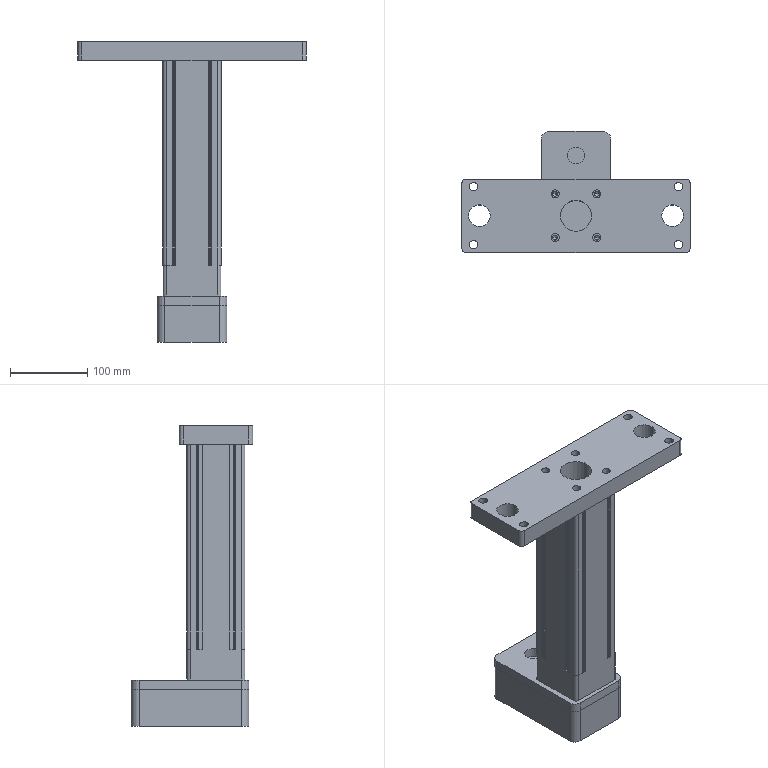Part | STEP file | Electric cylinder assembly 2 | 1 solid | 175 faces | box 295 x 157.01 x 389 mm | volume 2717250 mm3 | plane 115 | cylinder 52 | cone 8 | commonest cylinder face diameters 10 x12 6.5 x8 10.5 x8 11 x8 20 x4 20.02 x4